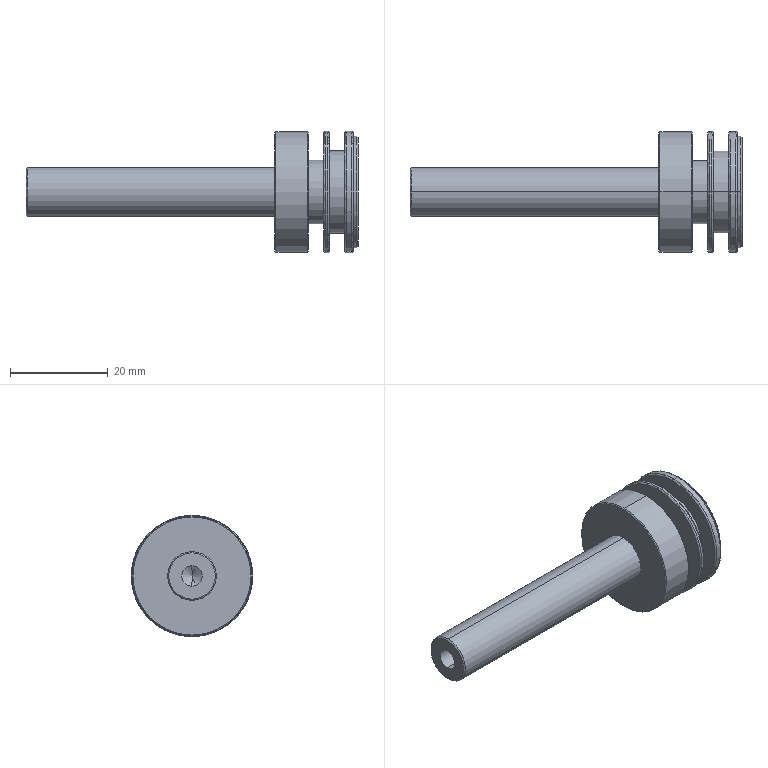Part | SolidWorks | features RefAxis 6, 3DProfileFeature 2, Revolution 2, HoleWzd 1 | 1 solid | 42 faces | box 68 x 24.9 x 24.9 mm | volume 9965 mm3 | cylinder 16 | cone 10 | torus 8 | plane 8 | commonest cylinder face diameters 24.9 x4 4.2 x2 10 x2 13 x2 16.9 x2 22.9 x2
STEP:
#1=CARTESIAN_POINT('',(-23.6,0.,-2.1));
#2=VERTEX_POINT('',#1);
#3=CARTESIAN_POINT('',(-23.6,0.,2.1));
#4=VERTEX_POINT('',#3);
#5=CARTESIAN_POINT('',(-23.6,0.,0.));
#6=DIRECTION('',(-1.,0.,0.));
#7=DIRECTION('',(0.,0.,1.));
#8=AXIS2_PLACEMENT_3D('',#5,#6,#7);
#9=CIRCLE('',#8,2.1);
#10=EDGE_CURVE('',#2,#4,#9,.T.);
#11=ORIENTED_EDGE('',*,*,#10,.F.);
#12=CARTESIAN_POINT('',(-36.,0.,-2.1));
#13=VERTEX_POINT('',#12);
#14=CARTESIAN_POINT('',(-36.,0.,-2.1));
#15=DIRECTION('',(-1.,0.,0.));
#16=VECTOR('',#15,1000.);
#17=LINE('',#14,#16);
#18=EDGE_CURVE('',#2,#13,#17,.T.);
#19=ORIENTED_EDGE('',*,*,#18,.T.);
#20=CARTESIAN_POINT('',(-36.,0.,2.1));
#21=VERTEX_POINT('',#20);
#22=CARTESIAN_POINT('',(-36.,0.,0.));
#23=DIRECTION('',(-1.,0.,0.));
#24=DIRECTION('',(0.,0.,1.));
#25=AXIS2_PLACEMENT_3D('',#22,#23,#24);
#26=CIRCLE('',#25,2.1);
#27=EDGE_CURVE('',#13,#21,#26,.T.);
#28=ORIENTED_EDGE('',*,*,#27,.T.);
#29=CARTESIAN_POINT('',(-36.,0.,2.1));
#30=DIRECTION('',(-1.,0.,0.));
#31=VECTOR('',#30,1000.);
#32=LINE('',#29,#31);
#33=EDGE_CURVE('',#4,#21,#32,.T.);
#34=ORIENTED_EDGE('',*,*,#33,.F.);
#35=EDGE_LOOP('',(#11,#19,#28,#34));
#36=FACE_OUTER_BOUND('',#35,.T.);
#37=CARTESIAN_POINT('',(-36.,0.,0.));
#38=DIRECTION('',(-1.,0.,0.));
#39=DIRECTION('',(0.,0.,1.));
#40=AXIS2_PLACEMENT_3D('',#37,#38,#39);
#41=CYLINDRICAL_SURFACE('',#40,2.1);
#42=ADVANCED_FACE('',(#36),#41,.F.);
#43=CARTESIAN_POINT('',(-22.338,0.,0.));
#44=VERTEX_POINT('',#43);
#45=CARTESIAN_POINT('',(-23.6,0.,2.1));
#46=DIRECTION('',(-0.515,0.,0.8572));
#47=VECTOR('',#46,1000.);
#48=LINE('',#45,#47);
#49=EDGE_CURVE('',#44,#4,#48,.T.);
#50=ORIENTED_EDGE('',*,*,#49,.F.);
#51=CARTESIAN_POINT('',(-23.6,0.,-2.1));
#52=DIRECTION('',(-0.515,0.,-0.8572));
#53=VECTOR('',#52,1000.);
#54=LINE('',#51,#53);
#55=EDGE_CURVE('',#44,#2,#54,.T.);
#56=ORIENTED_EDGE('',*,*,#55,.T.);
#57=ORIENTED_EDGE('',*,*,#10,.T.);
#58=EDGE_LOOP('',(#50,#56,#57));
#59=FACE_OUTER_BOUND('',#58,.T.);
#60=CARTESIAN_POINT('',(-23.6,0.,0.));
#61=DIRECTION('',(-1.,0.,0.));
#62=DIRECTION('',(0.,0.,1.));
#63=AXIS2_PLACEMENT_3D('',#60,#61,#62);
#64=CONICAL_SURFACE('',#63,2.1,1.03);
#65=ADVANCED_FACE('',(#59),#64,.F.);
#66=CARTESIAN_POINT('',(32.,0.,11.15));
#67=VERTEX_POINT('',#66);
#68=CARTESIAN_POINT('',(32.,0.,-11.15));
#69=VERTEX_POINT('',#68);
#70=CARTESIAN_POINT('',(32.,0.,0.));
#71=DIRECTION('',(-1.,0.,0.));
#72=DIRECTION('',(0.,0.,1.));
#73=AXIS2_PLACEMENT_3D('',#70,#71,#72);
#74=CIRCLE('',#73,11.15);
#75=EDGE_CURVE('',#67,#69,#74,.T.);
#76=ORIENTED_EDGE('',*,*,#75,.T.);
#77=CARTESIAN_POINT('',(31.7,0.,-11.45));
#78=VERTEX_POINT('',#77);
#79=CARTESIAN_POINT('',(32.,0.,-11.15));
#80=DIRECTION('',(-0.7071,0.,-0.7071));
#81=VECTOR('',#80,1000.);
#82=LINE('',#79,#81);
#83=EDGE_CURVE('',#69,#78,#82,.T.);
#84=ORIENTED_EDGE('',*,*,#83,.T.);
#85=CARTESIAN_POINT('',(31.7,0.,11.45));
#86=VERTEX_POINT('',#85);
#87=CARTESIAN_POINT('',(31.7,0.,0.));
#88=DIRECTION('',(-1.,0.,0.));
#89=DIRECTION('',(0.,0.,1.));
#90=AXIS2_PLACEMENT_3D('',#87,#88,#89);
#91=CIRCLE('',#90,11.45);
#92=EDGE_CURVE('',#86,#78,#91,.T.);
#93=ORIENTED_EDGE('',*,*,#92,.F.);
#94=CARTESIAN_POINT('',(32.,0.,11.15));
#95=DIRECTION('',(-0.7071,0.,0.7071));
#96=VECTOR('',#95,1000.);
#97=LINE('',#94,#96);
#98=EDGE_CURVE('',#67,#86,#97,.T.);
#99=ORIENTED_EDGE('',*,*,#98,.F.);
#100=EDGE_LOOP('',(#76,#84,#93,#99));
#101=FACE_OUTER_BOUND('',#100,.T.);
#102=CARTESIAN_POINT('',(32.,0.,0.));
#103=DIRECTION('',(-1.,0.,0.));
#104=DIRECTION('',(0.,0.,1.));
#105=AXIS2_PLACEMENT_3D('',#102,#103,#104);
#106=CONICAL_SURFACE('',#105,11.15,0.7854);
#107=ADVANCED_FACE('',(#101),#106,.T.);
#108=ORIENTED_EDGE('',*,*,#92,.T.);
#109=CARTESIAN_POINT('',(31.,0.,-11.45));
#110=VERTEX_POINT('',#109);
#111=CARTESIAN_POINT('',(32.,0.,-11.45));
#112=DIRECTION('',(-1.,0.,0.));
#113=VECTOR('',#112,1000.);
#114=LINE('',#111,#113);
#115=EDGE_CURVE('',#78,#110,#114,.T.);
#116=ORIENTED_EDGE('',*,*,#115,.T.);
#117=CARTESIAN_POINT('',(31.,0.,11.45));
#118=VERTEX_POINT('',#117);
#119=CARTESIAN_POINT('',(31.,0.,0.));
#120=DIRECTION('',(-1.,0.,0.));
#121=DIRECTION('',(0.,0.,1.));
#122=AXIS2_PLACEMENT_3D('',#119,#120,#121);
#123=CIRCLE('',#122,11.45);
#124=EDGE_CURVE('',#118,#110,#123,.T.);
#125=ORIENTED_EDGE('',*,*,#124,.F.);
#126=CARTESIAN_POINT('',(32.,0.,11.45));
#127=DIRECTION('',(-1.,0.,0.));
#128=VECTOR('',#127,1000.);
#129=LINE('',#126,#128);
#130=EDGE_CURVE('',#86,#118,#129,.T.);
#131=ORIENTED_EDGE('',*,*,#130,.F.);
#132=EDGE_LOOP('',(#108,#116,#125,#131));
#133=FACE_OUTER_BOUND('',#132,.T.);
#134=CARTESIAN_POINT('',(32.,0.,0.));
#135=DIRECTION('',(-1.,0.,0.));
#136=DIRECTION('',(0.,0.,1.));
#137=AXIS2_PLACEMENT_3D('',#134,#135,#136);
#138=CYLINDRICAL_SURFACE('',#137,11.45);
#139=ADVANCED_FACE('',(#133),#138,.T.);
#140=CARTESIAN_POINT('',(31.,0.,12.15));
#141=VERTEX_POINT('',#140);
#142=CARTESIAN_POINT('',(31.,0.,-12.15));
#143=VERTEX_POINT('',#142);
#144=CARTESIAN_POINT('',(31.,0.,0.));
#145=DIRECTION('',(-1.,0.,0.));
#146=DIRECTION('',(0.,0.,1.));
#147=AXIS2_PLACEMENT_3D('',#144,#145,#146);
#148=CIRCLE('',#147,12.15);
#149=EDGE_CURVE('',#141,#143,#148,.T.);
#150=ORIENTED_EDGE('',*,*,#149,.T.);
#151=CARTESIAN_POINT('',(30.7,0.,-12.45));
#152=VERTEX_POINT('',#151);
#153=CARTESIAN_POINT('',(30.7,0.,-12.15));
#154=DIRECTION('',(0.,1.,0.));
#155=DIRECTION('',(0.,0.,1.));
#156=AXIS2_PLACEMENT_3D('',#153,#154,#155);
#157=CIRCLE('',#156,0.3);
#158=EDGE_CURVE('',#143,#152,#157,.T.);
#159=ORIENTED_EDGE('',*,*,#158,.T.);
#160=CARTESIAN_POINT('',(30.7,0.,12.45));
#161=VERTEX_POINT('',#160);
#162=CARTESIAN_POINT('',(30.7,0.,0.));
#163=DIRECTION('',(-1.,0.,0.));
#164=DIRECTION('',(0.,0.,1.));
#165=AXIS2_PLACEMENT_3D('',#162,#163,#164);
#166=CIRCLE('',#165,12.45);
#167=EDGE_CURVE('',#161,#152,#166,.T.);
#168=ORIENTED_EDGE('',*,*,#167,.F.);
#169=CARTESIAN_POINT('',(30.7,0.,12.15));
#170=DIRECTION('',(0.,-1.,0.));
#171=DIRECTION('',(0.,0.,-1.));
#172=AXIS2_PLACEMENT_3D('',#169,#170,#171);
#173=CIRCLE('',#172,0.3);
#174=EDGE_CURVE('',#141,#161,#173,.T.);
#175=ORIENTED_EDGE('',*,*,#174,.F.);
#176=EDGE_LOOP('',(#150,#159,#168,#175));
#177=FACE_OUTER_BOUND('',#176,.T.);
#178=CARTESIAN_POINT('',(30.7,0.,0.));
#179=DIRECTION('',(-1.,0.,0.));
#180=DIRECTION('',(0.,0.,1.));
#181=AXIS2_PLACEMENT_3D('',#178,#179,#180);
#182=TOROIDAL_SURFACE('',#181,12.15,0.3);
#183=ADVANCED_FACE('',(#177),#182,.T.);
#184=ORIENTED_EDGE('',*,*,#167,.T.);
#185=CARTESIAN_POINT('',(29.6,0.,-12.45));
#186=VERTEX_POINT('',#185);
#187=CARTESIAN_POINT('',(32.,0.,-12.45));
#188=DIRECTION('',(-1.,0.,0.));
#189=VECTOR('',#188,1000.);
#190=LINE('',#187,#189);
#191=EDGE_CURVE('',#152,#186,#190,.T.);
#192=ORIENTED_EDGE('',*,*,#191,.T.);
#193=CARTESIAN_POINT('',(29.6,0.,12.45));
#194=VERTEX_POINT('',#193);
#195=CARTESIAN_POINT('',(29.6,0.,0.));
#196=DIRECTION('',(-1.,0.,0.));
#197=DIRECTION('',(0.,0.,1.));
#198=AXIS2_PLACEMENT_3D('',#195,#196,#197);
#199=CIRCLE('',#198,12.45);
#200=EDGE_CURVE('',#194,#186,#199,.T.);
#201=ORIENTED_EDGE('',*,*,#200,.F.);
#202=CARTESIAN_POINT('',(32.,0.,12.45));
#203=DIRECTION('',(-1.,0.,0.));
#204=VECTOR('',#203,1000.);
#205=LINE('',#202,#204);
#206=EDGE_CURVE('',#161,#194,#205,.T.);
#207=ORIENTED_EDGE('',*,*,#206,.F.);
#208=EDGE_LOOP('',(#184,#192,#201,#207));
#209=FACE_OUTER_BOUND('',#208,.T.);
#210=CARTESIAN_POINT('',(32.,0.,0.));
#211=DIRECTION('',(-1.,0.,0.));
#212=DIRECTION('',(0.,0.,1.));
#213=AXIS2_PLACEMENT_3D('',#210,#211,#212);
#214=CYLINDRICAL_SURFACE('',#213,12.45);
#215=ADVANCED_FACE('',(#209),#214,.T.);
#216=ORIENTED_EDGE('',*,*,#200,.T.);
#217=CARTESIAN_POINT('',(29.3,0.,-12.15));
#218=VERTEX_POINT('',#217);
#219=CARTESIAN_POINT('',(29.6,0.,-12.15));
#220=DIRECTION('',(0.,1.,0.));
#221=DIRECTION('',(0.,0.,1.));
#222=AXIS2_PLACEMENT_3D('',#219,#220,#221);
#223=CIRCLE('',#222,0.3);
#224=EDGE_CURVE('',#186,#218,#223,.T.);
#225=ORIENTED_EDGE('',*,*,#224,.T.);
#226=CARTESIAN_POINT('',(29.3,0.,12.15));
#227=VERTEX_POINT('',#226);
#228=CARTESIAN_POINT('',(29.3,0.,0.));
#229=DIRECTION('',(-1.,0.,0.));
#230=DIRECTION('',(0.,0.,1.));
#231=AXIS2_PLACEMENT_3D('',#228,#229,#230);
#232=CIRCLE('',#231,12.15);
#233=EDGE_CURVE('',#227,#218,#232,.T.);
#234=ORIENTED_EDGE('',*,*,#233,.F.);
#235=CARTESIAN_POINT('',(29.6,0.,12.15));
#236=DIRECTION('',(0.,-1.,0.));
#237=DIRECTION('',(0.,0.,-1.));
#238=AXIS2_PLACEMENT_3D('',#235,#236,#237);
#239=CIRCLE('',#238,0.3);
#240=EDGE_CURVE('',#194,#227,#239,.T.);
#241=ORIENTED_EDGE('',*,*,#240,.F.);
#242=EDGE_LOOP('',(#216,#225,#234,#241));
#243=FACE_OUTER_BOUND('',#242,.T.);
#244=CARTESIAN_POINT('',(29.6,0.,0.));
#245=DIRECTION('',(-1.,0.,0.));
#246=DIRECTION('',(0.,0.,1.));
#247=AXIS2_PLACEMENT_3D('',#244,#245,#246);
#248=TOROIDAL_SURFACE('',#247,12.15,0.3);
#249=ADVANCED_FACE('',(#243),#248,.T.);
#250=CARTESIAN_POINT('',(29.3,0.,8.45));
#251=VERTEX_POINT('',#250);
#252=CARTESIAN_POINT('',(29.3,0.,-8.45));
#253=VERTEX_POINT('',#252);
#254=CARTESIAN_POINT('',(29.3,0.,0.));
#255=DIRECTION('',(-1.,0.,0.));
#256=DIRECTION('',(0.,0.,1.));
#257=AXIS2_PLACEMENT_3D('',#254,#255,#256);
#258=CIRCLE('',#257,8.45);
#259=EDGE_CURVE('',#251,#253,#258,.T.);
#260=ORIENTED_EDGE('',*,*,#259,.T.);
#261=CARTESIAN_POINT('',(26.1,0.,-8.45));
#262=VERTEX_POINT('',#261);
#263=CARTESIAN_POINT('',(32.,0.,-8.45));
#264=DIRECTION('',(-1.,0.,0.));
#265=VECTOR('',#264,1000.);
#266=LINE('',#263,#265);
#267=EDGE_CURVE('',#253,#262,#266,.T.);
#268=ORIENTED_EDGE('',*,*,#267,.T.);
#269=CARTESIAN_POINT('',(26.1,0.,8.45));
#270=VERTEX_POINT('',#269);
#271=CARTESIAN_POINT('',(26.1,0.,0.));
#272=DIRECTION('',(-1.,0.,0.));
#273=DIRECTION('',(0.,0.,1.));
#274=AXIS2_PLACEMENT_3D('',#271,#272,#273);
#275=CIRCLE('',#274,8.45);
#276=EDGE_CURVE('',#270,#262,#275,.T.);
#277=ORIENTED_EDGE('',*,*,#276,.F.);
#278=CARTESIAN_POINT('',(32.,0.,8.45));
#279=DIRECTION('',(-1.,0.,0.));
#280=VECTOR('',#279,1000.);
#281=LINE('',#278,#280);
#282=EDGE_CURVE('',#251,#270,#281,.T.);
#283=ORIENTED_EDGE('',*,*,#282,.F.);
#284=EDGE_LOOP('',(#260,#268,#277,#283));
#285=FACE_OUTER_BOUND('',#284,.T.);
#286=CARTESIAN_POINT('',(32.,0.,0.));
#287=DIRECTION('',(-1.,0.,0.));
#288=DIRECTION('',(0.,0.,1.));
#289=AXIS2_PLACEMENT_3D('',#286,#287,#288);
#290=CYLINDRICAL_SURFACE('',#289,8.45);
#291=ADVANCED_FACE('',(#285),#290,.T.);
#292=CARTESIAN_POINT('',(26.1,0.,12.15));
#293=VERTEX_POINT('',#292);
#294=CARTESIAN_POINT('',(26.1,0.,-12.15));
#295=VERTEX_POINT('',#294);
#296=CARTESIAN_POINT('',(26.1,0.,0.));
#297=DIRECTION('',(-1.,0.,0.));
#298=DIRECTION('',(0.,0.,1.));
#299=AXIS2_PLACEMENT_3D('',#296,#297,#298);
#300=CIRCLE('',#299,12.15);
#301=EDGE_CURVE('',#293,#295,#300,.T.);
#302=ORIENTED_EDGE('',*,*,#301,.T.);
#303=CARTESIAN_POINT('',(25.8,0.,-12.45));
#304=VERTEX_POINT('',#303);
#305=CARTESIAN_POINT('',(25.8,0.,-12.15));
#306=DIRECTION('',(0.,1.,0.));
#307=DIRECTION('',(0.,0.,1.));
#308=AXIS2_PLACEMENT_3D('',#305,#306,#307);
#309=CIRCLE('',#308,0.3);
#310=EDGE_CURVE('',#295,#304,#309,.T.);
#311=ORIENTED_EDGE('',*,*,#310,.T.);
#312=CARTESIAN_POINT('',(25.8,0.,12.45));
#313=VERTEX_POINT('',#312);
#314=CARTESIAN_POINT('',(25.8,0.,0.));
#315=DIRECTION('',(-1.,0.,0.));
#316=DIRECTION('',(0.,0.,1.));
#317=AXIS2_PLACEMENT_3D('',#314,#315,#316);
#318=CIRCLE('',#317,12.45);
#319=EDGE_CURVE('',#313,#304,#318,.T.);
#320=ORIENTED_EDGE('',*,*,#319,.F.);
#321=CARTESIAN_POINT('',(25.8,0.,12.15));
#322=DIRECTION('',(0.,-1.,0.));
#323=DIRECTION('',(0.,0.,-1.));
#324=AXIS2_PLACEMENT_3D('',#321,#322,#323);
#325=CIRCLE('',#324,0.3);
#326=EDGE_CURVE('',#293,#313,#325,.T.);
#327=ORIENTED_EDGE('',*,*,#326,.F.);
#328=EDGE_LOOP('',(#302,#311,#320,#327));
#329=FACE_OUTER_BOUND('',#328,.T.);
#330=CARTESIAN_POINT('',(25.8,0.,0.));
#331=DIRECTION('',(-1.,0.,0.));
#332=DIRECTION('',(0.,0.,1.));
#333=AXIS2_PLACEMENT_3D('',#330,#331,#332);
#334=TOROIDAL_SURFACE('',#333,12.15,0.3);
#335=ADVANCED_FACE('',(#329),#334,.T.);
#336=ORIENTED_EDGE('',*,*,#319,.T.);
#337=CARTESIAN_POINT('',(25.3,0.,-12.45));
#338=VERTEX_POINT('',#337);
#339=CARTESIAN_POINT('',(32.,0.,-12.45));
#340=DIRECTION('',(-1.,0.,0.));
#341=VECTOR('',#340,1000.);
#342=LINE('',#339,#341);
#343=EDGE_CURVE('',#304,#338,#342,.T.);
#344=ORIENTED_EDGE('',*,*,#343,.T.);
#345=CARTESIAN_POINT('',(25.3,0.,12.45));
#346=VERTEX_POINT('',#345);
#347=CARTESIAN_POINT('',(25.3,0.,0.));
#348=DIRECTION('',(-1.,0.,0.));
#349=DIRECTION('',(0.,0.,1.));
#350=AXIS2_PLACEMENT_3D('',#347,#348,#349);
#351=CIRCLE('',#350,12.45);
#352=EDGE_CURVE('',#346,#338,#351,.T.);
#353=ORIENTED_EDGE('',*,*,#352,.F.);
#354=CARTESIAN_POINT('',(32.,0.,12.45));
#355=DIRECTION('',(-1.,0.,0.));
#356=VECTOR('',#355,1000.);
#357=LINE('',#354,#356);
#358=EDGE_CURVE('',#313,#346,#357,.T.);
#359=ORIENTED_EDGE('',*,*,#358,.F.);
#360=EDGE_LOOP('',(#336,#344,#353,#359));
#361=FACE_OUTER_BOUND('',#360,.T.);
#362=CARTESIAN_POINT('',(32.,0.,0.));
#363=DIRECTION('',(-1.,0.,0.));
#364=DIRECTION('',(0.,0.,1.));
#365=AXIS2_PLACEMENT_3D('',#362,#363,#364);
#366=CYLINDRICAL_SURFACE('',#365,12.45);
#367=ADVANCED_FACE('',(#361),#366,.T.);
#368=ORIENTED_EDGE('',*,*,#352,.T.);
#369=CARTESIAN_POINT('',(25.,0.,-12.15));
#370=VERTEX_POINT('',#369);
#371=CARTESIAN_POINT('',(25.3,0.,-12.15));
#372=DIRECTION('',(0.,1.,0.));
#373=DIRECTION('',(0.,0.,1.));
#374=AXIS2_PLACEMENT_3D('',#371,#372,#373);
#375=CIRCLE('',#374,0.3);
#376=EDGE_CURVE('',#338,#370,#375,.T.);
#377=ORIENTED_EDGE('',*,*,#376,.T.);
#378=CARTESIAN_POINT('',(25.,0.,12.15));
#379=VERTEX_POINT('',#378);
#380=CARTESIAN_POINT('',(25.,0.,0.));
#381=DIRECTION('',(-1.,0.,0.));
#382=DIRECTION('',(0.,0.,1.));
#383=AXIS2_PLACEMENT_3D('',#380,#381,#382);
#384=CIRCLE('',#383,12.15);
#385=EDGE_CURVE('',#379,#370,#384,.T.);
#386=ORIENTED_EDGE('',*,*,#385,.F.);
#387=CARTESIAN_POINT('',(25.3,0.,12.15));
#388=DIRECTION('',(0.,-1.,0.));
#389=DIRECTION('',(0.,0.,-1.));
#390=AXIS2_PLACEMENT_3D('',#387,#388,#389);
#391=CIRCLE('',#390,0.3);
#392=EDGE_CURVE('',#346,#379,#391,.T.);
#393=ORIENTED_EDGE('',*,*,#392,.F.);
#394=EDGE_LOOP('',(#368,#377,#386,#393));
#395=FACE_OUTER_BOUND('',#394,.T.);
#396=CARTESIAN_POINT('',(25.3,0.,0.));
#397=DIRECTION('',(-1.,0.,0.));
#398=DIRECTION('',(0.,0.,1.));
#399=AXIS2_PLACEMENT_3D('',#396,#397,#398);
#400=TOROIDAL_SURFACE('',#399,12.15,0.3);
#401=ADVANCED_FACE('',(#395),#400,.T.);
#402=CARTESIAN_POINT('',(25.,0.,6.5));
#403=VERTEX_POINT('',#402);
#404=CARTESIAN_POINT('',(25.,0.,-6.5));
#405=VERTEX_POINT('',#404);
#406=CARTESIAN_POINT('',(25.,0.,0.));
#407=DIRECTION('',(-1.,0.,0.));
#408=DIRECTION('',(0.,0.,1.));
#409=AXIS2_PLACEMENT_3D('',#406,#407,#408);
#410=CIRCLE('',#409,6.5);
#411=EDGE_CURVE('',#403,#405,#410,.T.);
#412=ORIENTED_EDGE('',*,*,#411,.T.);
#413=CARTESIAN_POINT('',(21.8,0.,-6.5));
#414=VERTEX_POINT('',#413);
#415=CARTESIAN_POINT('',(32.,0.,-6.5));
#416=DIRECTION('',(-1.,0.,0.));
#417=VECTOR('',#416,1000.);
#418=LINE('',#415,#417);
#419=EDGE_CURVE('',#405,#414,#418,.T.);
#420=ORIENTED_EDGE('',*,*,#419,.T.);
#421=CARTESIAN_POINT('',(21.8,0.,6.5));
#422=VERTEX_POINT('',#421);
#423=CARTESIAN_POINT('',(21.8,0.,0.));
#424=DIRECTION('',(-1.,0.,0.));
#425=DIRECTION('',(0.,0.,1.));
#426=AXIS2_PLACEMENT_3D('',#423,#424,#425);
#427=CIRCLE('',#426,6.5);
#428=EDGE_CURVE('',#422,#414,#427,.T.);
#429=ORIENTED_EDGE('',*,*,#428,.F.);
#430=CARTESIAN_POINT('',(32.,0.,6.5));
#431=DIRECTION('',(-1.,0.,0.));
#432=VECTOR('',#431,1000.);
#433=LINE('',#430,#432);
#434=EDGE_CURVE('',#403,#422,#433,.T.);
#435=ORIENTED_EDGE('',*,*,#434,.F.);
#436=EDGE_LOOP('',(#412,#420,#429,#435));
#437=FACE_OUTER_BOUND('',#436,.T.);
#438=CARTESIAN_POINT('',(32.,0.,0.));
#439=DIRECTION('',(-1.,0.,0.));
#440=DIRECTION('',(0.,0.,1.));
#441=AXIS2_PLACEMENT_3D('',#438,#439,#440);
#442=CYLINDRICAL_SURFACE('',#441,6.5);
#443=ADVANCED_FACE('',(#437),#442,.T.);
#444=CARTESIAN_POINT('',(21.8,0.,12.1));
#445=VERTEX_POINT('',#444);
#446=CARTESIAN_POINT('',(21.8,0.,-12.1));
#447=VERTEX_POINT('',#446);
#448=CARTESIAN_POINT('',(21.8,0.,0.));
#449=DIRECTION('',(-1.,0.,0.));
#450=DIRECTION('',(0.,0.,1.));
#451=AXIS2_PLACEMENT_3D('',#448,#449,#450);
#452=CIRCLE('',#451,12.1);
#453=EDGE_CURVE('',#445,#447,#452,.T.);
#454=ORIENTED_EDGE('',*,*,#453,.T.);
#455=CARTESIAN_POINT('',(21.6,0.,-12.3));
#456=VERTEX_POINT('',#455);
#457=CARTESIAN_POINT('',(21.8,0.,-12.1));
#458=DIRECTION('',(-0.7071,0.,-0.7071));
#459=VECTOR('',#458,1000.);
#460=LINE('',#457,#459);
#461=EDGE_CURVE('',#447,#456,#460,.T.);
#462=ORIENTED_EDGE('',*,*,#461,.T.);
#463=CARTESIAN_POINT('',(21.6,0.,12.3));
#464=VERTEX_POINT('',#463);
#465=CARTESIAN_POINT('',(21.6,0.,0.));
#466=DIRECTION('',(-1.,0.,0.));
#467=DIRECTION('',(0.,0.,1.));
#468=AXIS2_PLACEMENT_3D('',#465,#466,#467);
#469=CIRCLE('',#468,12.3);
#470=EDGE_CURVE('',#464,#456,#469,.T.);
#471=ORIENTED_EDGE('',*,*,#470,.F.);
#472=CARTESIAN_POINT('',(21.8,0.,12.1));
#473=DIRECTION('',(-0.7071,0.,0.7071));
#474=VECTOR('',#473,1000.);
#475=LINE('',#472,#474);
#476=EDGE_CURVE('',#445,#464,#475,.T.);
#477=ORIENTED_EDGE('',*,*,#476,.F.);
#478=EDGE_LOOP('',(#454,#462,#471,#477));
#479=FACE_OUTER_BOUND('',#478,.T.);
#480=CARTESIAN_POINT('',(21.8,0.,0.));
#481=DIRECTION('',(-1.,0.,0.));
#482=DIRECTION('',(0.,0.,1.));
#483=AXIS2_PLACEMENT_3D('',#480,#481,#482);
#484=CONICAL_SURFACE('',#483,12.1,0.7854);
#485=ADVANCED_FACE('',(#479),#484,.T.);
#486=ORIENTED_EDGE('',*,*,#470,.T.);
#487=CARTESIAN_POINT('',(15.2,0.,-12.3));
#488=VERTEX_POINT('',#487);
#489=CARTESIAN_POINT('',(32.,0.,-12.3));
#490=DIRECTION('',(-1.,0.,0.));
#491=VECTOR('',#490,1000.);
#492=LINE('',#489,#491);
#493=EDGE_CURVE('',#456,#488,#492,.T.);
#494=ORIENTED_EDGE('',*,*,#493,.T.);
#495=CARTESIAN_POINT('',(15.2,0.,12.3));
#496=VERTEX_POINT('',#495);
#497=CARTESIAN_POINT('',(15.2,0.,0.));
#498=DIRECTION('',(-1.,0.,0.));
#499=DIRECTION('',(0.,0.,1.));
#500=AXIS2_PLACEMENT_3D('',#497,#498,#499);
#501=CIRCLE('',#500,12.3);
#502=EDGE_CURVE('',#496,#488,#501,.T.);
#503=ORIENTED_EDGE('',*,*,#502,.F.);
#504=CARTESIAN_POINT('',(32.,0.,12.3));
#505=DIRECTION('',(-1.,0.,0.));
#506=VECTOR('',#505,1000.);
#507=LINE('',#504,#506);
#508=EDGE_CURVE('',#464,#496,#507,.T.);
#509=ORIENTED_EDGE('',*,*,#508,.F.);
#510=EDGE_LOOP('',(#486,#494,#503,#509));
#511=FACE_OUTER_BOUND('',#510,.T.);
#512=CARTESIAN_POINT('',(32.,0.,0.));
#513=DIRECTION('',(-1.,0.,0.));
#514=DIRECTION('',(0.,0.,1.));
#515=AXIS2_PLACEMENT_3D('',#512,#513,#514);
#516=CYLINDRICAL_SURFACE('',#515,12.3);
#517=ADVANCED_FACE('',(#511),#516,.T.);
#518=CARTESIAN_POINT('',(15.,0.,12.1));
#519=VERTEX_POINT('',#518);
#520=CARTESIAN_POINT('',(15.,0.,-12.1));
#521=VERTEX_POINT('',#520);
#522=CARTESIAN_POINT('',(15.,0.,0.));
#523=DIRECTION('',(-1.,0.,0.));
#524=DIRECTION('',(0.,0.,1.));
#525=AXIS2_PLACEMENT_3D('',#522,#523,#524);
#526=CIRCLE('',#525,12.1);
#527=EDGE_CURVE('',#519,#521,#526,.T.);
#528=ORIENTED_EDGE('',*,*,#527,.F.);
#529=CARTESIAN_POINT('',(15.2,0.,12.3));
#530=DIRECTION('',(0.7071,0.,0.7071));
#531=VECTOR('',#530,1000.);
#532=LINE('',#529,#531);
#533=EDGE_CURVE('',#519,#496,#532,.T.);
#534=ORIENTED_EDGE('',*,*,#533,.T.);
#535=ORIENTED_EDGE('',*,*,#502,.T.);
#536=CARTESIAN_POINT('',(15.2,0.,-12.3));
#537=DIRECTION('',(0.7071,0.,-0.7071));
#538=VECTOR('',#537,1000.);
#539=LINE('',#536,#538);
#540=EDGE_CURVE('',#521,#488,#539,.T.);
#541=ORIENTED_EDGE('',*,*,#540,.F.);
#542=EDGE_LOOP('',(#528,#534,#535,#541));
#543=FACE_OUTER_BOUND('',#542,.T.);
#544=CARTESIAN_POINT('',(15.2,0.,0.));
#545=DIRECTION('',(1.,0.,0.));
#546=DIRECTION('',(0.,0.,-1.));
#547=AXIS2_PLACEMENT_3D('',#544,#545,#546);
#548=CONICAL_SURFACE('',#547,12.3,0.7854);
#549=ADVANCED_FACE('',(#543),#548,.T.);
#550=CARTESIAN_POINT('',(15.,0.,5.));
#551=VERTEX_POINT('',#550);
#552=CARTESIAN_POINT('',(15.,0.,-5.));
#553=VERTEX_POINT('',#552);
#554=CARTESIAN_POINT('',(15.,0.,0.));
#555=DIRECTION('',(-1.,0.,0.));
#556=DIRECTION('',(0.,0.,1.));
#557=AXIS2_PLACEMENT_3D('',#554,#555,#556);
#558=CIRCLE('',#557,5.);
#559=EDGE_CURVE('',#551,#553,#558,.T.);
#560=ORIENTED_EDGE('',*,*,#559,.T.);
#561=CARTESIAN_POINT('',(-35.75,0.,-5.));
#562=VERTEX_POINT('',#561);
#563=CARTESIAN_POINT('',(0.,0.,-5.));
#564=DIRECTION('',(-1.,0.,0.));
#565=VECTOR('',#564,1000.);
#566=LINE('',#563,#565);
#567=EDGE_CURVE('',#553,#562,#566,.T.);
#568=ORIENTED_EDGE('',*,*,#567,.T.);
#569=CARTESIAN_POINT('',(-35.75,0.,5.));
#570=VERTEX_POINT('',#569);
#571=CARTESIAN_POINT('',(-35.75,0.,0.));
#572=DIRECTION('',(-1.,0.,0.));
#573=DIRECTION('',(0.,0.,1.));
#574=AXIS2_PLACEMENT_3D('',#571,#572,#573);
#575=CIRCLE('',#574,5.);
#576=EDGE_CURVE('',#570,#562,#575,.T.);
#577=ORIENTED_EDGE('',*,*,#576,.F.);
#578=CARTESIAN_POINT('',(0.,0.,5.));
#579=DIRECTION('',(-1.,0.,0.));
#580=VECTOR('',#579,1000.);
#581=LINE('',#578,#580);
#582=EDGE_CURVE('',#551,#570,#581,.T.);
#583=ORIENTED_EDGE('',*,*,#582,.F.);
#584=EDGE_LOOP('',(#560,#568,#577,#583));
#585=FACE_OUTER_BOUND('',#584,.T.);
#586=CARTESIAN_POINT('',(0.,0.,0.));
#587=DIRECTION('',(-1.,0.,0.));
#588=DIRECTION('',(0.,0.,1.));
#589=AXIS2_PLACEMENT_3D('',#586,#587,#588);
#590=CYLINDRICAL_SURFACE('',#589,5.);
#591=ADVANCED_FACE('',(#585),#590,.T.);
#592=CARTESIAN_POINT('',(-36.,0.,4.75));
#593=VERTEX_POINT('',#592);
#594=CARTESIAN_POINT('',(-36.,0.,-4.75));
#595=VERTEX_POINT('',#594);
#596=CARTESIAN_POINT('',(-36.,0.,0.));
#597=DIRECTION('',(-1.,0.,0.));
#598=DIRECTION('',(0.,0.,1.));
#599=AXIS2_PLACEMENT_3D('',#596,#597,#598);
#600=CIRCLE('',#599,4.75);
#601=EDGE_CURVE('',#593,#595,#600,.T.);
#602=ORIENTED_EDGE('',*,*,#601,.F.);
#603=CARTESIAN_POINT('',(-35.75,0.,5.));
#604=DIRECTION('',(0.7071,0.,0.7071));
#605=VECTOR('',#604,1000.);
#606=LINE('',#603,#605);
#607=EDGE_CURVE('',#593,#570,#606,.T.);
#608=ORIENTED_EDGE('',*,*,#607,.T.);
#609=ORIENTED_EDGE('',*,*,#576,.T.);
#610=CARTESIAN_POINT('',(-35.75,0.,-5.));
#611=DIRECTION('',(0.7071,0.,-0.7071));
#612=VECTOR('',#611,1000.);
#613=LINE('',#610,#612);
#614=EDGE_CURVE('',#595,#562,#613,.T.);
#615=ORIENTED_EDGE('',*,*,#614,.F.);
#616=EDGE_LOOP('',(#602,#608,#609,#615));
#617=FACE_OUTER_BOUND('',#616,.T.);
#618=CARTESIAN_POINT('',(-35.75,0.,0.));
#619=DIRECTION('',(1.,0.,0.));
#620=DIRECTION('',(0.,0.,-1.));
#621=AXIS2_PLACEMENT_3D('',#618,#619,#620);
#622=CONICAL_SURFACE('',#621,5.,0.7854);
#623=ADVANCED_FACE('',(#617),#622,.T.);
#624=CARTESIAN_POINT('',(-36.,0.,0.));
#625=DIRECTION('',(-1.,0.,0.));
#626=DIRECTION('',(0.,0.,1.));
#627=AXIS2_PLACEMENT_3D('',#624,#625,#626);
#628=CIRCLE('',#627,2.1);
#629=EDGE_CURVE('',#21,#13,#628,.T.);
#630=ORIENTED_EDGE('',*,*,#629,.F.);
#631=ORIENTED_EDGE('',*,*,#27,.F.);
#632=EDGE_LOOP('',(#630,#631));
#633=FACE_BOUND('',#632,.T.);
#634=CARTESIAN_POINT('',(-36.,0.,0.));
#635=DIRECTION('',(-1.,0.,0.));
#636=DIRECTION('',(0.,0.,1.));
#637=AXIS2_PLACEMENT_3D('',#634,#635,#636);
#638=CIRCLE('',#637,4.75);
#639=EDGE_CURVE('',#595,#593,#638,.T.);
#640=ORIENTED_EDGE('',*,*,#639,.T.);
#641=ORIENTED_EDGE('',*,*,#601,.T.);
#642=EDGE_LOOP('',(#640,#641));
#643=FACE_OUTER_BOUND('',#642,.T.);
#644=CARTESIAN_POINT('',(-36.,0.,0.));
#645=DIRECTION('',(1.,0.,0.));
#646=DIRECTION('',(0.,0.,-1.));
#647=AXIS2_PLACEMENT_3D('',#644,#645,#646);
#648=PLANE('',#647);
#649=ADVANCED_FACE('',(#633,#643),#648,.F.);
#650=ORIENTED_EDGE('',*,*,#607,.F.);
#651=ORIENTED_EDGE('',*,*,#639,.F.);
#652=ORIENTED_EDGE('',*,*,#614,.T.);
#653=CARTESIAN_POINT('',(-35.75,0.,0.));
#654=DIRECTION('',(-1.,0.,0.));
#655=DIRECTION('',(0.,0.,1.));
#656=AXIS2_PLACEMENT_3D('',#653,#654,#655);
#657=CIRCLE('',#656,5.);
#658=EDGE_CURVE('',#562,#570,#657,.T.);
#659=ORIENTED_EDGE('',*,*,#658,.T.);
#660=EDGE_LOOP('',(#650,#651,#652,#659));
#661=FACE_OUTER_BOUND('',#660,.T.);
#662=CARTESIAN_POINT('',(-35.75,0.,0.));
#663=DIRECTION('',(1.,0.,0.));
#664=DIRECTION('',(0.,0.,-1.));
#665=AXIS2_PLACEMENT_3D('',#662,#663,#664);
#666=CONICAL_SURFACE('',#665,5.,0.7854);
#667=ADVANCED_FACE('',(#661),#666,.T.);
#668=ORIENTED_EDGE('',*,*,#567,.F.);
#669=CARTESIAN_POINT('',(15.,0.,0.));
#670=DIRECTION('',(-1.,0.,0.));
#671=DIRECTION('',(0.,0.,1.));
#672=AXIS2_PLACEMENT_3D('',#669,#670,#671);
#673=CIRCLE('',#672,5.);
#674=EDGE_CURVE('',#553,#551,#673,.T.);
#675=ORIENTED_EDGE('',*,*,#674,.T.);
#676=ORIENTED_EDGE('',*,*,#582,.T.);
#677=ORIENTED_EDGE('',*,*,#658,.F.);
#678=EDGE_LOOP('',(#668,#675,#676,#677));
#679=FACE_OUTER_BOUND('',#678,.T.);
#680=CARTESIAN_POINT('',(0.,0.,0.));
#681=DIRECTION('',(-1.,0.,0.));
#682=DIRECTION('',(0.,0.,1.));
#683=AXIS2_PLACEMENT_3D('',#680,#681,#682);
#684=CYLINDRICAL_SURFACE('',#683,5.);
#685=ADVANCED_FACE('',(#679),#684,.T.);
#686=ORIENTED_EDGE('',*,*,#559,.F.);
#687=ORIENTED_EDGE('',*,*,#674,.F.);
#688=EDGE_LOOP('',(#686,#687));
#689=FACE_BOUND('',#688,.T.);
#690=CARTESIAN_POINT('',(15.,0.,0.));
#691=DIRECTION('',(-1.,0.,0.));
#692=DIRECTION('',(0.,0.,1.));
#693=AXIS2_PLACEMENT_3D('',#690,#691,#692);
#694=CIRCLE('',#693,12.1);
#695=EDGE_CURVE('',#521,#519,#694,.T.);
#696=ORIENTED_EDGE('',*,*,#695,.T.);
#697=ORIENTED_EDGE('',*,*,#527,.T.);
#698=EDGE_LOOP('',(#696,#697));
#699=FACE_OUTER_BOUND('',#698,.T.);
#700=CARTESIAN_POINT('',(15.,5.,0.));
#701=DIRECTION('',(1.,0.,0.));
#702=DIRECTION('',(0.,0.,-1.));
#703=AXIS2_PLACEMENT_3D('',#700,#701,#702);
#704=PLANE('',#703);
#705=ADVANCED_FACE('',(#689,#699),#704,.F.);
#706=ORIENTED_EDGE('',*,*,#533,.F.);
#707=ORIENTED_EDGE('',*,*,#695,.F.);
#708=ORIENTED_EDGE('',*,*,#540,.T.);
#709=CARTESIAN_POINT('',(15.2,0.,0.));
#710=DIRECTION('',(-1.,0.,0.));
#711=DIRECTION('',(0.,0.,1.));
#712=AXIS2_PLACEMENT_3D('',#709,#710,#711);
#713=CIRCLE('',#712,12.3);
#714=EDGE_CURVE('',#488,#496,#713,.T.);
#715=ORIENTED_EDGE('',*,*,#714,.T.);
#716=EDGE_LOOP('',(#706,#707,#708,#715));
#717=FACE_OUTER_BOUND('',#716,.T.);
#718=CARTESIAN_POINT('',(15.2,0.,0.));
#719=DIRECTION('',(1.,0.,0.));
#720=DIRECTION('',(0.,0.,-1.));
#721=AXIS2_PLACEMENT_3D('',#718,#719,#720);
#722=CONICAL_SURFACE('',#721,12.3,0.7854);
#723=ADVANCED_FACE('',(#717),#722,.T.);
#724=ORIENTED_EDGE('',*,*,#493,.F.);
#725=CARTESIAN_POINT('',(21.6,0.,0.));
#726=DIRECTION('',(-1.,0.,0.));
#727=DIRECTION('',(0.,0.,1.));
#728=AXIS2_PLACEMENT_3D('',#725,#726,#727);
#729=CIRCLE('',#728,12.3);
#730=EDGE_CURVE('',#456,#464,#729,.T.);
#731=ORIENTED_EDGE('',*,*,#730,.T.);
#732=ORIENTED_EDGE('',*,*,#508,.T.);
#733=ORIENTED_EDGE('',*,*,#714,.F.);
#734=EDGE_LOOP('',(#724,#731,#732,#733));
#735=FACE_OUTER_BOUND('',#734,.T.);
#736=CARTESIAN_POINT('',(32.,0.,0.));
#737=DIRECTION('',(-1.,0.,0.));
#738=DIRECTION('',(0.,0.,1.));
#739=AXIS2_PLACEMENT_3D('',#736,#737,#738);
#740=CYLINDRICAL_SURFACE('',#739,12.3);
#741=ADVANCED_FACE('',(#735),#740,.T.);
#742=ORIENTED_EDGE('',*,*,#461,.F.);
#743=CARTESIAN_POINT('',(21.8,0.,0.));
#744=DIRECTION('',(-1.,0.,0.));
#745=DIRECTION('',(0.,0.,1.));
#746=AXIS2_PLACEMENT_3D('',#743,#744,#745);
#747=CIRCLE('',#746,12.1);
#748=EDGE_CURVE('',#447,#445,#747,.T.);
#749=ORIENTED_EDGE('',*,*,#748,.T.);
#750=ORIENTED_EDGE('',*,*,#476,.T.);
#751=ORIENTED_EDGE('',*,*,#730,.F.);
#752=EDGE_LOOP('',(#742,#749,#750,#751));
#753=FACE_OUTER_BOUND('',#752,.T.);
#754=CARTESIAN_POINT('',(21.8,0.,0.));
#755=DIRECTION('',(-1.,0.,0.));
#756=DIRECTION('',(0.,0.,1.));
#757=AXIS2_PLACEMENT_3D('',#754,#755,#756);
#758=CONICAL_SURFACE('',#757,12.1,0.7854);
#759=ADVANCED_FACE('',(#753),#758,.T.);
#760=ORIENTED_EDGE('',*,*,#453,.F.);
#761=ORIENTED_EDGE('',*,*,#748,.F.);
#762=EDGE_LOOP('',(#760,#761));
#763=FACE_OUTER_BOUND('',#762,.T.);
#764=ORIENTED_EDGE('',*,*,#428,.T.);
#765=CARTESIAN_POINT('',(21.8,0.,0.));
#766=DIRECTION('',(-1.,0.,0.));
#767=DIRECTION('',(0.,0.,1.));
#768=AXIS2_PLACEMENT_3D('',#765,#766,#767);
#769=CIRCLE('',#768,6.5);
#770=EDGE_CURVE('',#414,#422,#769,.T.);
#771=ORIENTED_EDGE('',*,*,#770,.T.);
#772=EDGE_LOOP('',(#764,#771));
#773=FACE_BOUND('',#772,.T.);
#774=CARTESIAN_POINT('',(21.8,12.1,0.));
#775=DIRECTION('',(-1.,0.,0.));
#776=DIRECTION('',(0.,0.,1.));
#777=AXIS2_PLACEMENT_3D('',#774,#775,#776);
#778=PLANE('',#777);
#779=ADVANCED_FACE('',(#763,#773),#778,.F.);
#780=ORIENTED_EDGE('',*,*,#419,.F.);
#781=CARTESIAN_POINT('',(25.,0.,0.));
#782=DIRECTION('',(-1.,0.,0.));
#783=DIRECTION('',(0.,0.,1.));
#784=AXIS2_PLACEMENT_3D('',#781,#782,#783);
#785=CIRCLE('',#784,6.5);
#786=EDGE_CURVE('',#405,#403,#785,.T.);
#787=ORIENTED_EDGE('',*,*,#786,.T.);
#788=ORIENTED_EDGE('',*,*,#434,.T.);
#789=ORIENTED_EDGE('',*,*,#770,.F.);
#790=EDGE_LOOP('',(#780,#787,#788,#789));
#791=FACE_OUTER_BOUND('',#790,.T.);
#792=CARTESIAN_POINT('',(32.,0.,0.));
#793=DIRECTION('',(-1.,0.,0.));
#794=DIRECTION('',(0.,0.,1.));
#795=AXIS2_PLACEMENT_3D('',#792,#793,#794);
#796=CYLINDRICAL_SURFACE('',#795,6.5);
#797=ADVANCED_FACE('',(#791),#796,.T.);
#798=ORIENTED_EDGE('',*,*,#411,.F.);
#799=ORIENTED_EDGE('',*,*,#786,.F.);
#800=EDGE_LOOP('',(#798,#799));
#801=FACE_BOUND('',#800,.T.);
#802=ORIENTED_EDGE('',*,*,#385,.T.);
#803=CARTESIAN_POINT('',(25.,0.,0.));
#804=DIRECTION('',(-1.,0.,0.));
#805=DIRECTION('',(0.,0.,1.));
#806=AXIS2_PLACEMENT_3D('',#803,#804,#805);
#807=CIRCLE('',#806,12.15);
#808=EDGE_CURVE('',#370,#379,#807,.T.);
#809=ORIENTED_EDGE('',*,*,#808,.T.);
#810=EDGE_LOOP('',(#802,#809));
#811=FACE_OUTER_BOUND('',#810,.T.);
#812=CARTESIAN_POINT('',(25.,6.5,0.));
#813=DIRECTION('',(1.,0.,0.));
#814=DIRECTION('',(0.,0.,-1.));
#815=AXIS2_PLACEMENT_3D('',#812,#813,#814);
#816=PLANE('',#815);
#817=ADVANCED_FACE('',(#801,#811),#816,.F.);
#818=ORIENTED_EDGE('',*,*,#376,.F.);
#819=CARTESIAN_POINT('',(25.3,0.,0.));
#820=DIRECTION('',(-1.,0.,0.));
#821=DIRECTION('',(0.,0.,1.));
#822=AXIS2_PLACEMENT_3D('',#819,#820,#821);
#823=CIRCLE('',#822,12.45);
#824=EDGE_CURVE('',#338,#346,#823,.T.);
#825=ORIENTED_EDGE('',*,*,#824,.T.);
#826=ORIENTED_EDGE('',*,*,#392,.T.);
#827=ORIENTED_EDGE('',*,*,#808,.F.);
#828=EDGE_LOOP('',(#818,#825,#826,#827));
#829=FACE_OUTER_BOUND('',#828,.T.);
#830=CARTESIAN_POINT('',(25.3,0.,0.));
#831=DIRECTION('',(-1.,0.,0.));
#832=DIRECTION('',(0.,0.,1.));
#833=AXIS2_PLACEMENT_3D('',#830,#831,#832);
#834=TOROIDAL_SURFACE('',#833,12.15,0.3);
#835=ADVANCED_FACE('',(#829),#834,.T.);
#836=ORIENTED_EDGE('',*,*,#343,.F.);
#837=CARTESIAN_POINT('',(25.8,0.,0.));
#838=DIRECTION('',(-1.,0.,0.));
#839=DIRECTION('',(0.,0.,1.));
#840=AXIS2_PLACEMENT_3D('',#837,#838,#839);
#841=CIRCLE('',#840,12.45);
#842=EDGE_CURVE('',#304,#313,#841,.T.);
#843=ORIENTED_EDGE('',*,*,#842,.T.);
#844=ORIENTED_EDGE('',*,*,#358,.T.);
#845=ORIENTED_EDGE('',*,*,#824,.F.);
#846=EDGE_LOOP('',(#836,#843,#844,#845));
#847=FACE_OUTER_BOUND('',#846,.T.);
#848=CARTESIAN_POINT('',(32.,0.,0.));
#849=DIRECTION('',(-1.,0.,0.));
#850=DIRECTION('',(0.,0.,1.));
#851=AXIS2_PLACEMENT_3D('',#848,#849,#850);
#852=CYLINDRICAL_SURFACE('',#851,12.45);
#853=ADVANCED_FACE('',(#847),#852,.T.);
#854=ORIENTED_EDGE('',*,*,#310,.F.);
#855=CARTESIAN_POINT('',(26.1,0.,0.));
#856=DIRECTION('',(-1.,0.,0.));
#857=DIRECTION('',(0.,0.,1.));
#858=AXIS2_PLACEMENT_3D('',#855,#856,#857);
#859=CIRCLE('',#858,12.15);
#860=EDGE_CURVE('',#295,#293,#859,.T.);
#861=ORIENTED_EDGE('',*,*,#860,.T.);
#862=ORIENTED_EDGE('',*,*,#326,.T.);
#863=ORIENTED_EDGE('',*,*,#842,.F.);
#864=EDGE_LOOP('',(#854,#861,#862,#863));
#865=FACE_OUTER_BOUND('',#864,.T.);
#866=CARTESIAN_POINT('',(25.8,0.,0.));
#867=DIRECTION('',(-1.,0.,0.));
#868=DIRECTION('',(0.,0.,1.));
#869=AXIS2_PLACEMENT_3D('',#866,#867,#868);
#870=TOROIDAL_SURFACE('',#869,12.15,0.3);
#871=ADVANCED_FACE('',(#865),#870,.T.);
#872=ORIENTED_EDGE('',*,*,#301,.F.);
#873=ORIENTED_EDGE('',*,*,#860,.F.);
#874=EDGE_LOOP('',(#872,#873));
#875=FACE_OUTER_BOUND('',#874,.T.);
#876=ORIENTED_EDGE('',*,*,#276,.T.);
#877=CARTESIAN_POINT('',(26.1,0.,0.));
#878=DIRECTION('',(-1.,0.,0.));
#879=DIRECTION('',(0.,0.,1.));
#880=AXIS2_PLACEMENT_3D('',#877,#878,#879);
#881=CIRCLE('',#880,8.45);
#882=EDGE_CURVE('',#262,#270,#881,.T.);
#883=ORIENTED_EDGE('',*,*,#882,.T.);
#884=EDGE_LOOP('',(#876,#883));
#885=FACE_BOUND('',#884,.T.);
#886=CARTESIAN_POINT('',(26.1,12.15,0.));
#887=DIRECTION('',(-1.,0.,0.));
#888=DIRECTION('',(0.,0.,1.));
#889=AXIS2_PLACEMENT_3D('',#886,#887,#888);
#890=PLANE('',#889);
#891=ADVANCED_FACE('',(#875,#885),#890,.F.);
#892=ORIENTED_EDGE('',*,*,#267,.F.);
#893=CARTESIAN_POINT('',(29.3,0.,0.));
#894=DIRECTION('',(-1.,0.,0.));
#895=DIRECTION('',(0.,0.,1.));
#896=AXIS2_PLACEMENT_3D('',#893,#894,#895);
#897=CIRCLE('',#896,8.45);
#898=EDGE_CURVE('',#253,#251,#897,.T.);
#899=ORIENTED_EDGE('',*,*,#898,.T.);
#900=ORIENTED_EDGE('',*,*,#282,.T.);
#901=ORIENTED_EDGE('',*,*,#882,.F.);
#902=EDGE_LOOP('',(#892,#899,#900,#901));
#903=FACE_OUTER_BOUND('',#902,.T.);
#904=CARTESIAN_POINT('',(32.,0.,0.));
#905=DIRECTION('',(-1.,0.,0.));
#906=DIRECTION('',(0.,0.,1.));
#907=AXIS2_PLACEMENT_3D('',#904,#905,#906);
#908=CYLINDRICAL_SURFACE('',#907,8.45);
#909=ADVANCED_FACE('',(#903),#908,.T.);
#910=ORIENTED_EDGE('',*,*,#259,.F.);
#911=ORIENTED_EDGE('',*,*,#898,.F.);
#912=EDGE_LOOP('',(#910,#911));
#913=FACE_BOUND('',#912,.T.);
#914=ORIENTED_EDGE('',*,*,#233,.T.);
#915=CARTESIAN_POINT('',(29.3,0.,0.));
#916=DIRECTION('',(-1.,0.,0.));
#917=DIRECTION('',(0.,0.,1.));
#918=AXIS2_PLACEMENT_3D('',#915,#916,#917);
#919=CIRCLE('',#918,12.15);
#920=EDGE_CURVE('',#218,#227,#919,.T.);
#921=ORIENTED_EDGE('',*,*,#920,.T.);
#922=EDGE_LOOP('',(#914,#921));
#923=FACE_OUTER_BOUND('',#922,.T.);
#924=CARTESIAN_POINT('',(29.3,8.45,0.));
#925=DIRECTION('',(1.,0.,0.));
#926=DIRECTION('',(0.,0.,-1.));
#927=AXIS2_PLACEMENT_3D('',#924,#925,#926);
#928=PLANE('',#927);
#929=ADVANCED_FACE('',(#913,#923),#928,.F.);
#930=ORIENTED_EDGE('',*,*,#224,.F.);
#931=CARTESIAN_POINT('',(29.6,0.,0.));
#932=DIRECTION('',(-1.,0.,0.));
#933=DIRECTION('',(0.,0.,1.));
#934=AXIS2_PLACEMENT_3D('',#931,#932,#933);
#935=CIRCLE('',#934,12.45);
#936=EDGE_CURVE('',#186,#194,#935,.T.);
#937=ORIENTED_EDGE('',*,*,#936,.T.);
#938=ORIENTED_EDGE('',*,*,#240,.T.);
#939=ORIENTED_EDGE('',*,*,#920,.F.);
#940=EDGE_LOOP('',(#930,#937,#938,#939));
#941=FACE_OUTER_BOUND('',#940,.T.);
#942=CARTESIAN_POINT('',(29.6,0.,0.));
#943=DIRECTION('',(-1.,0.,0.));
#944=DIRECTION('',(0.,0.,1.));
#945=AXIS2_PLACEMENT_3D('',#942,#943,#944);
#946=TOROIDAL_SURFACE('',#945,12.15,0.3);
#947=ADVANCED_FACE('',(#941),#946,.T.);
#948=ORIENTED_EDGE('',*,*,#191,.F.);
#949=CARTESIAN_POINT('',(30.7,0.,0.));
#950=DIRECTION('',(-1.,0.,0.));
#951=DIRECTION('',(0.,0.,1.));
#952=AXIS2_PLACEMENT_3D('',#949,#950,#951);
#953=CIRCLE('',#952,12.45);
#954=EDGE_CURVE('',#152,#161,#953,.T.);
#955=ORIENTED_EDGE('',*,*,#954,.T.);
#956=ORIENTED_EDGE('',*,*,#206,.T.);
#957=ORIENTED_EDGE('',*,*,#936,.F.);
#958=EDGE_LOOP('',(#948,#955,#956,#957));
#959=FACE_OUTER_BOUND('',#958,.T.);
#960=CARTESIAN_POINT('',(32.,0.,0.));
#961=DIRECTION('',(-1.,0.,0.));
#962=DIRECTION('',(0.,0.,1.));
#963=AXIS2_PLACEMENT_3D('',#960,#961,#962);
#964=CYLINDRICAL_SURFACE('',#963,12.45);
#965=ADVANCED_FACE('',(#959),#964,.T.);
#966=ORIENTED_EDGE('',*,*,#158,.F.);
#967=CARTESIAN_POINT('',(31.,0.,0.));
#968=DIRECTION('',(-1.,0.,0.));
#969=DIRECTION('',(0.,0.,1.));
#970=AXIS2_PLACEMENT_3D('',#967,#968,#969);
#971=CIRCLE('',#970,12.15);
#972=EDGE_CURVE('',#143,#141,#971,.T.);
#973=ORIENTED_EDGE('',*,*,#972,.T.);
#974=ORIENTED_EDGE('',*,*,#174,.T.);
#975=ORIENTED_EDGE('',*,*,#954,.F.);
#976=EDGE_LOOP('',(#966,#973,#974,#975));
#977=FACE_OUTER_BOUND('',#976,.T.);
#978=CARTESIAN_POINT('',(30.7,0.,0.));
#979=DIRECTION('',(-1.,0.,0.));
#980=DIRECTION('',(0.,0.,1.));
#981=AXIS2_PLACEMENT_3D('',#978,#979,#980);
#982=TOROIDAL_SURFACE('',#981,12.15,0.3);
#983=ADVANCED_FACE('',(#977),#982,.T.);
#984=ORIENTED_EDGE('',*,*,#149,.F.);
#985=ORIENTED_EDGE('',*,*,#972,.F.);
#986=EDGE_LOOP('',(#984,#985));
#987=FACE_OUTER_BOUND('',#986,.T.);
#988=ORIENTED_EDGE('',*,*,#124,.T.);
#989=CARTESIAN_POINT('',(31.,0.,0.));
#990=DIRECTION('',(-1.,0.,0.));
#991=DIRECTION('',(0.,0.,1.));
#992=AXIS2_PLACEMENT_3D('',#989,#990,#991);
#993=CIRCLE('',#992,11.45);
#994=EDGE_CURVE('',#110,#118,#993,.T.);
#995=ORIENTED_EDGE('',*,*,#994,.T.);
#996=EDGE_LOOP('',(#988,#995));
#997=FACE_BOUND('',#996,.T.);
#998=CARTESIAN_POINT('',(31.,12.15,0.));
#999=DIRECTION('',(-1.,0.,0.));
#1000=DIRECTION('',(0.,0.,1.));
#1001=AXIS2_PLACEMENT_3D('',#998,#999,#1000);
#1002=PLANE('',#1001);
#1003=ADVANCED_FACE('',(#987,#997),#1002,.F.);
#1004=ORIENTED_EDGE('',*,*,#115,.F.);
#1005=CARTESIAN_POINT('',(31.7,0.,0.));
#1006=DIRECTION('',(-1.,0.,0.));
#1007=DIRECTION('',(0.,0.,1.));
#1008=AXIS2_PLACEMENT_3D('',#1005,#1006,#1007);
#1009=CIRCLE('',#1008,11.45);
#1010=EDGE_CURVE('',#78,#86,#1009,.T.);
#1011=ORIENTED_EDGE('',*,*,#1010,.T.);
#1012=ORIENTED_EDGE('',*,*,#130,.T.);
#1013=ORIENTED_EDGE('',*,*,#994,.F.);
#1014=EDGE_LOOP('',(#1004,#1011,#1012,#1013));
#1015=FACE_OUTER_BOUND('',#1014,.T.);
#1016=CARTESIAN_POINT('',(32.,0.,0.));
#1017=DIRECTION('',(-1.,0.,0.));
#1018=DIRECTION('',(0.,0.,1.));
#1019=AXIS2_PLACEMENT_3D('',#1016,#1017,#1018);
#1020=CYLINDRICAL_SURFACE('',#1019,11.45);
#1021=ADVANCED_FACE('',(#1015),#1020,.T.);
#1022=ORIENTED_EDGE('',*,*,#83,.F.);
#1023=CARTESIAN_POINT('',(32.,0.,0.));
#1024=DIRECTION('',(-1.,0.,0.));
#1025=DIRECTION('',(0.,0.,1.));
#1026=AXIS2_PLACEMENT_3D('',#1023,#1024,#1025);
#1027=CIRCLE('',#1026,11.15);
#1028=EDGE_CURVE('',#69,#67,#1027,.T.);
#1029=ORIENTED_EDGE('',*,*,#1028,.T.);
#1030=ORIENTED_EDGE('',*,*,#98,.T.);
#1031=ORIENTED_EDGE('',*,*,#1010,.F.);
#1032=EDGE_LOOP('',(#1022,#1029,#1030,#1031));
#1033=FACE_OUTER_BOUND('',#1032,.T.);
#1034=CARTESIAN_POINT('',(32.,0.,0.));
#1035=DIRECTION('',(-1.,0.,0.));
#1036=DIRECTION('',(0.,0.,1.));
#1037=AXIS2_PLACEMENT_3D('',#1034,#1035,#1036);
#1038=CONICAL_SURFACE('',#1037,11.15,0.7854);
#1039=ADVANCED_FACE('',(#1033),#1038,.T.);
#1040=ORIENTED_EDGE('',*,*,#75,.F.);
#1041=ORIENTED_EDGE('',*,*,#1028,.F.);
#1042=EDGE_LOOP('',(#1040,#1041));
#1043=FACE_OUTER_BOUND('',#1042,.T.);
#1044=CARTESIAN_POINT('',(32.,11.15,0.));
#1045=DIRECTION('',(-1.,0.,0.));
#1046=DIRECTION('',(0.,0.,1.));
#1047=AXIS2_PLACEMENT_3D('',#1044,#1045,#1046);
#1048=PLANE('',#1047);
#1049=ADVANCED_FACE('',(#1043),#1048,.F.);
#1050=ORIENTED_EDGE('',*,*,#55,.F.);
#1051=ORIENTED_EDGE('',*,*,#49,.T.);
#1052=CARTESIAN_POINT('',(-23.6,0.,0.));
#1053=DIRECTION('',(-1.,0.,0.));
#1054=DIRECTION('',(0.,0.,1.));
#1055=AXIS2_PLACEMENT_3D('',#1052,#1053,#1054);
#1056=CIRCLE('',#1055,2.1);
#1057=EDGE_CURVE('',#4,#2,#1056,.T.);
#1058=ORIENTED_EDGE('',*,*,#1057,.T.);
#1059=EDGE_LOOP('',(#1050,#1051,#1058));
#1060=FACE_OUTER_BOUND('',#1059,.T.);
#1061=CARTESIAN_POINT('',(-23.6,0.,0.));
#1062=DIRECTION('',(-1.,0.,0.));
#1063=DIRECTION('',(0.,0.,1.));
#1064=AXIS2_PLACEMENT_3D('',#1061,#1062,#1063);
#1065=CONICAL_SURFACE('',#1064,2.1,1.03);
#1066=ADVANCED_FACE('',(#1060),#1065,.F.);
#1067=ORIENTED_EDGE('',*,*,#18,.F.);
#1068=ORIENTED_EDGE('',*,*,#1057,.F.);
#1069=ORIENTED_EDGE('',*,*,#33,.T.);
#1070=ORIENTED_EDGE('',*,*,#629,.T.);
#1071=EDGE_LOOP('',(#1067,#1068,#1069,#1070));
#1072=FACE_OUTER_BOUND('',#1071,.T.);
#1073=CARTESIAN_POINT('',(-36.,0.,0.));
#1074=DIRECTION('',(-1.,0.,0.));
#1075=DIRECTION('',(0.,0.,1.));
#1076=AXIS2_PLACEMENT_3D('',#1073,#1074,#1075);
#1077=CYLINDRICAL_SURFACE('',#1076,2.1);
#1078=ADVANCED_FACE('',(#1072),#1077,.F.);
#1079=CLOSED_SHELL('',(#42,#65,#107,#139,#183,#215,#249,#291,#335,#367,#401,#443,#485,#517,#549,#591,#623,#649,#667,#685,#705,#723,#741,#759,#779,#797,#817,#835,#853,#871,#891,#909,#929,#947,#965,#983,#1003,#1021,#1039,#1049,#1066,#1078));
#1080=MANIFOLD_SOLID_BREP('',#1079);
#1081=CARTESIAN_POINT('',(0.,0.,0.));
#1082=DIRECTION('',(0.,0.,1.));
#1083=DIRECTION('',(1.,0.,0.));
#1084=AXIS2_PLACEMENT_3D('',#1081,#1082,#1083);
#1085=(LENGTH_UNIT()NAMED_UNIT(*)SI_UNIT(.MILLI.,.METRE.));
#1086=UNCERTAINTY_MEASURE_WITH_UNIT(LENGTH_MEASURE(0.00001),#1085,'','');
#1087=(NAMED_UNIT(*)PLANE_ANGLE_UNIT()SI_UNIT($,.RADIAN.));
#1088=(NAMED_UNIT(*)SI_UNIT($,.STERADIAN.)SOLID_ANGLE_UNIT());
#1089=(GEOMETRIC_REPRESENTATION_CONTEXT(3)GLOBAL_UNCERTAINTY_ASSIGNED_CONTEXT((#1086))GLOBAL_UNIT_ASSIGNED_CONTEXT((#1085,#1087,#1088))REPRESENTATION_CONTEXT('',''));
#1090=ADVANCED_BREP_SHAPE_REPRESENTATION('',(#1080,#1084),#1089);